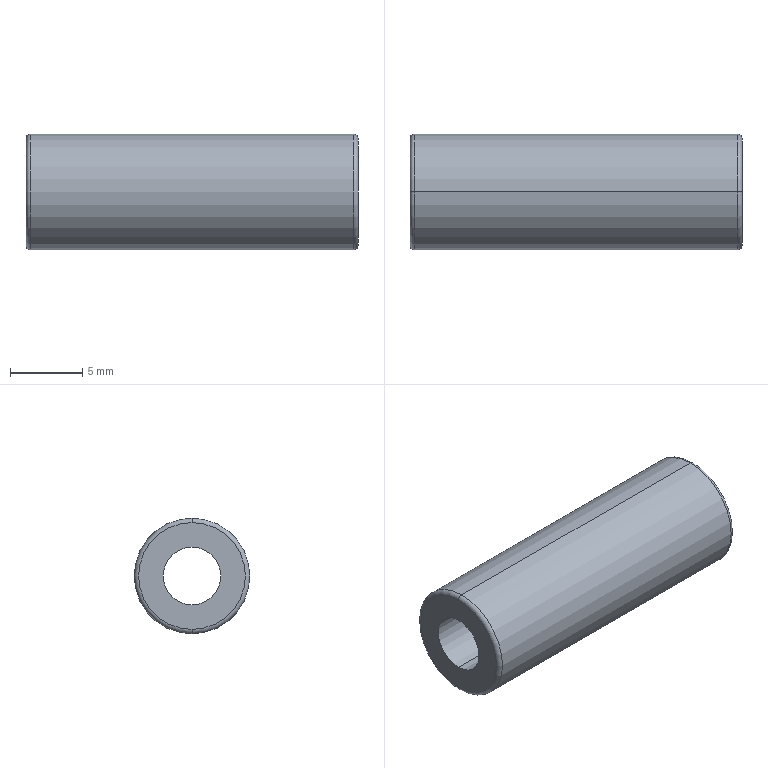Part | SolidWorks | features RefAxis 3, 3DProfileFeature 1, Revolution 1 | 1 solid | 10 faces | box 23 x 8 x 8 mm | volume 866.125 mm3 | torus 4 | cylinder 4 | plane 2 | commonest cylinder face diameters 4 x2 8 x2
STEP:
#1=CARTESIAN_POINT('',(0.3,0.,4.));
#2=VERTEX_POINT('',#1);
#3=CARTESIAN_POINT('',(0.3,0.,-4.));
#4=VERTEX_POINT('',#3);
#5=CARTESIAN_POINT('',(0.3,0.,0.));
#6=DIRECTION('',(-1.,0.,0.));
#7=DIRECTION('',(0.,0.,1.));
#8=AXIS2_PLACEMENT_3D('',#5,#6,#7);
#9=CIRCLE('',#8,4.);
#10=EDGE_CURVE('',#2,#4,#9,.T.);
#11=ORIENTED_EDGE('',*,*,#10,.T.);
#12=CARTESIAN_POINT('',(0.,0.,-3.7));
#13=VERTEX_POINT('',#12);
#14=CARTESIAN_POINT('',(0.3,0.,-3.7));
#15=DIRECTION('',(0.,1.,0.));
#16=DIRECTION('',(0.,0.,1.));
#17=AXIS2_PLACEMENT_3D('',#14,#15,#16);
#18=CIRCLE('',#17,0.3);
#19=EDGE_CURVE('',#4,#13,#18,.T.);
#20=ORIENTED_EDGE('',*,*,#19,.T.);
#21=CARTESIAN_POINT('',(0.,0.,3.7));
#22=VERTEX_POINT('',#21);
#23=CARTESIAN_POINT('',(0.,0.,0.));
#24=DIRECTION('',(-1.,0.,0.));
#25=DIRECTION('',(0.,0.,1.));
#26=AXIS2_PLACEMENT_3D('',#23,#24,#25);
#27=CIRCLE('',#26,3.7);
#28=EDGE_CURVE('',#22,#13,#27,.T.);
#29=ORIENTED_EDGE('',*,*,#28,.F.);
#30=CARTESIAN_POINT('',(0.3,0.,3.7));
#31=DIRECTION('',(0.,-1.,0.));
#32=DIRECTION('',(0.,0.,-1.));
#33=AXIS2_PLACEMENT_3D('',#30,#31,#32);
#34=CIRCLE('',#33,0.3);
#35=EDGE_CURVE('',#2,#22,#34,.T.);
#36=ORIENTED_EDGE('',*,*,#35,.F.);
#37=EDGE_LOOP('',(#11,#20,#29,#36));
#38=FACE_OUTER_BOUND('',#37,.T.);
#39=CARTESIAN_POINT('',(0.3,0.,0.));
#40=DIRECTION('',(-1.,0.,0.));
#41=DIRECTION('',(0.,0.,1.));
#42=AXIS2_PLACEMENT_3D('',#39,#40,#41);
#43=TOROIDAL_SURFACE('',#42,3.7,0.3);
#44=ADVANCED_FACE('',(#38),#43,.T.);
#45=CARTESIAN_POINT('',(22.7,0.,4.));
#46=VERTEX_POINT('',#45);
#47=CARTESIAN_POINT('',(22.7,0.,-4.));
#48=VERTEX_POINT('',#47);
#49=CARTESIAN_POINT('',(22.7,0.,0.));
#50=DIRECTION('',(-1.,0.,0.));
#51=DIRECTION('',(0.,0.,1.));
#52=AXIS2_PLACEMENT_3D('',#49,#50,#51);
#53=CIRCLE('',#52,4.);
#54=EDGE_CURVE('',#46,#48,#53,.T.);
#55=ORIENTED_EDGE('',*,*,#54,.T.);
#56=CARTESIAN_POINT('',(50.,0.,-4.));
#57=DIRECTION('',(-1.,0.,0.));
#58=VECTOR('',#57,1000.);
#59=LINE('',#56,#58);
#60=EDGE_CURVE('',#48,#4,#59,.T.);
#61=ORIENTED_EDGE('',*,*,#60,.T.);
#62=ORIENTED_EDGE('',*,*,#10,.F.);
#63=CARTESIAN_POINT('',(50.,0.,4.));
#64=DIRECTION('',(-1.,0.,0.));
#65=VECTOR('',#64,1000.);
#66=LINE('',#63,#65);
#67=EDGE_CURVE('',#46,#2,#66,.T.);
#68=ORIENTED_EDGE('',*,*,#67,.F.);
#69=EDGE_LOOP('',(#55,#61,#62,#68));
#70=FACE_OUTER_BOUND('',#69,.T.);
#71=CARTESIAN_POINT('',(50.,0.,0.));
#72=DIRECTION('',(-1.,0.,0.));
#73=DIRECTION('',(0.,0.,1.));
#74=AXIS2_PLACEMENT_3D('',#71,#72,#73);
#75=CYLINDRICAL_SURFACE('',#74,4.);
#76=ADVANCED_FACE('',(#70),#75,.T.);
#77=CARTESIAN_POINT('',(23.,0.,3.7));
#78=VERTEX_POINT('',#77);
#79=CARTESIAN_POINT('',(23.,0.,-3.7));
#80=VERTEX_POINT('',#79);
#81=CARTESIAN_POINT('',(23.,0.,0.));
#82=DIRECTION('',(-1.,0.,0.));
#83=DIRECTION('',(0.,0.,1.));
#84=AXIS2_PLACEMENT_3D('',#81,#82,#83);
#85=CIRCLE('',#84,3.7);
#86=EDGE_CURVE('',#78,#80,#85,.T.);
#87=ORIENTED_EDGE('',*,*,#86,.T.);
#88=CARTESIAN_POINT('',(22.7,0.,-3.7));
#89=DIRECTION('',(0.,1.,0.));
#90=DIRECTION('',(0.,0.,1.));
#91=AXIS2_PLACEMENT_3D('',#88,#89,#90);
#92=CIRCLE('',#91,0.3);
#93=EDGE_CURVE('',#80,#48,#92,.T.);
#94=ORIENTED_EDGE('',*,*,#93,.T.);
#95=ORIENTED_EDGE('',*,*,#54,.F.);
#96=CARTESIAN_POINT('',(22.7,0.,3.7));
#97=DIRECTION('',(0.,-1.,0.));
#98=DIRECTION('',(0.,0.,-1.));
#99=AXIS2_PLACEMENT_3D('',#96,#97,#98);
#100=CIRCLE('',#99,0.3);
#101=EDGE_CURVE('',#78,#46,#100,.T.);
#102=ORIENTED_EDGE('',*,*,#101,.F.);
#103=EDGE_LOOP('',(#87,#94,#95,#102));
#104=FACE_OUTER_BOUND('',#103,.T.);
#105=CARTESIAN_POINT('',(22.7,0.,0.));
#106=DIRECTION('',(-1.,0.,0.));
#107=DIRECTION('',(0.,0.,1.));
#108=AXIS2_PLACEMENT_3D('',#105,#106,#107);
#109=TOROIDAL_SURFACE('',#108,3.7,0.3);
#110=ADVANCED_FACE('',(#104),#109,.T.);
#111=CARTESIAN_POINT('',(23.,0.,-2.));
#112=VERTEX_POINT('',#111);
#113=CARTESIAN_POINT('',(23.,0.,2.));
#114=VERTEX_POINT('',#113);
#115=CARTESIAN_POINT('',(23.,0.,0.));
#116=DIRECTION('',(-1.,0.,0.));
#117=DIRECTION('',(0.,0.,1.));
#118=AXIS2_PLACEMENT_3D('',#115,#116,#117);
#119=CIRCLE('',#118,2.);
#120=EDGE_CURVE('',#112,#114,#119,.T.);
#121=ORIENTED_EDGE('',*,*,#120,.F.);
#122=CARTESIAN_POINT('',(0.,0.,-2.));
#123=VERTEX_POINT('',#122);
#124=CARTESIAN_POINT('',(50.,0.,-2.));
#125=DIRECTION('',(-1.,0.,0.));
#126=VECTOR('',#125,1000.);
#127=LINE('',#124,#126);
#128=EDGE_CURVE('',#112,#123,#127,.T.);
#129=ORIENTED_EDGE('',*,*,#128,.T.);
#130=CARTESIAN_POINT('',(0.,0.,2.));
#131=VERTEX_POINT('',#130);
#132=CARTESIAN_POINT('',(0.,0.,0.));
#133=DIRECTION('',(-1.,0.,0.));
#134=DIRECTION('',(0.,0.,1.));
#135=AXIS2_PLACEMENT_3D('',#132,#133,#134);
#136=CIRCLE('',#135,2.);
#137=EDGE_CURVE('',#123,#131,#136,.T.);
#138=ORIENTED_EDGE('',*,*,#137,.T.);
#139=CARTESIAN_POINT('',(50.,0.,2.));
#140=DIRECTION('',(-1.,0.,0.));
#141=VECTOR('',#140,1000.);
#142=LINE('',#139,#141);
#143=EDGE_CURVE('',#114,#131,#142,.T.);
#144=ORIENTED_EDGE('',*,*,#143,.F.);
#145=EDGE_LOOP('',(#121,#129,#138,#144));
#146=FACE_OUTER_BOUND('',#145,.T.);
#147=CARTESIAN_POINT('',(50.,0.,0.));
#148=DIRECTION('',(-1.,0.,0.));
#149=DIRECTION('',(0.,0.,1.));
#150=AXIS2_PLACEMENT_3D('',#147,#148,#149);
#151=CYLINDRICAL_SURFACE('',#150,2.);
#152=ADVANCED_FACE('',(#146),#151,.F.);
#153=CARTESIAN_POINT('',(0.,0.,0.));
#154=DIRECTION('',(-1.,0.,0.));
#155=DIRECTION('',(0.,0.,1.));
#156=AXIS2_PLACEMENT_3D('',#153,#154,#155);
#157=CIRCLE('',#156,2.);
#158=EDGE_CURVE('',#131,#123,#157,.T.);
#159=ORIENTED_EDGE('',*,*,#158,.F.);
#160=ORIENTED_EDGE('',*,*,#137,.F.);
#161=EDGE_LOOP('',(#159,#160));
#162=FACE_BOUND('',#161,.T.);
#163=ORIENTED_EDGE('',*,*,#28,.T.);
#164=CARTESIAN_POINT('',(0.,0.,0.));
#165=DIRECTION('',(-1.,0.,0.));
#166=DIRECTION('',(0.,0.,1.));
#167=AXIS2_PLACEMENT_3D('',#164,#165,#166);
#168=CIRCLE('',#167,3.7);
#169=EDGE_CURVE('',#13,#22,#168,.T.);
#170=ORIENTED_EDGE('',*,*,#169,.T.);
#171=EDGE_LOOP('',(#163,#170));
#172=FACE_OUTER_BOUND('',#171,.T.);
#173=CARTESIAN_POINT('',(0.,3.7,0.));
#174=DIRECTION('',(1.,0.,0.));
#175=DIRECTION('',(0.,0.,-1.));
#176=AXIS2_PLACEMENT_3D('',#173,#174,#175);
#177=PLANE('',#176);
#178=ADVANCED_FACE('',(#162,#172),#177,.F.);
#179=ORIENTED_EDGE('',*,*,#128,.F.);
#180=CARTESIAN_POINT('',(23.,0.,0.));
#181=DIRECTION('',(-1.,0.,0.));
#182=DIRECTION('',(0.,0.,1.));
#183=AXIS2_PLACEMENT_3D('',#180,#181,#182);
#184=CIRCLE('',#183,2.);
#185=EDGE_CURVE('',#114,#112,#184,.T.);
#186=ORIENTED_EDGE('',*,*,#185,.F.);
#187=ORIENTED_EDGE('',*,*,#143,.T.);
#188=ORIENTED_EDGE('',*,*,#158,.T.);
#189=EDGE_LOOP('',(#179,#186,#187,#188));
#190=FACE_OUTER_BOUND('',#189,.T.);
#191=CARTESIAN_POINT('',(50.,0.,0.));
#192=DIRECTION('',(-1.,0.,0.));
#193=DIRECTION('',(0.,0.,1.));
#194=AXIS2_PLACEMENT_3D('',#191,#192,#193);
#195=CYLINDRICAL_SURFACE('',#194,2.);
#196=ADVANCED_FACE('',(#190),#195,.F.);
#197=ORIENTED_EDGE('',*,*,#86,.F.);
#198=CARTESIAN_POINT('',(23.,0.,0.));
#199=DIRECTION('',(-1.,0.,0.));
#200=DIRECTION('',(0.,0.,1.));
#201=AXIS2_PLACEMENT_3D('',#198,#199,#200);
#202=CIRCLE('',#201,3.7);
#203=EDGE_CURVE('',#80,#78,#202,.T.);
#204=ORIENTED_EDGE('',*,*,#203,.F.);
#205=EDGE_LOOP('',(#197,#204));
#206=FACE_OUTER_BOUND('',#205,.T.);
#207=ORIENTED_EDGE('',*,*,#185,.T.);
#208=ORIENTED_EDGE('',*,*,#120,.T.);
#209=EDGE_LOOP('',(#207,#208));
#210=FACE_BOUND('',#209,.T.);
#211=CARTESIAN_POINT('',(23.,2.,0.));
#212=DIRECTION('',(-1.,0.,0.));
#213=DIRECTION('',(0.,0.,1.));
#214=AXIS2_PLACEMENT_3D('',#211,#212,#213);
#215=PLANE('',#214);
#216=ADVANCED_FACE('',(#206,#210),#215,.F.);
#217=ORIENTED_EDGE('',*,*,#93,.F.);
#218=ORIENTED_EDGE('',*,*,#203,.T.);
#219=ORIENTED_EDGE('',*,*,#101,.T.);
#220=CARTESIAN_POINT('',(22.7,0.,0.));
#221=DIRECTION('',(-1.,0.,0.));
#222=DIRECTION('',(0.,0.,1.));
#223=AXIS2_PLACEMENT_3D('',#220,#221,#222);
#224=CIRCLE('',#223,4.);
#225=EDGE_CURVE('',#48,#46,#224,.T.);
#226=ORIENTED_EDGE('',*,*,#225,.F.);
#227=EDGE_LOOP('',(#217,#218,#219,#226));
#228=FACE_OUTER_BOUND('',#227,.T.);
#229=CARTESIAN_POINT('',(22.7,0.,0.));
#230=DIRECTION('',(-1.,0.,0.));
#231=DIRECTION('',(0.,0.,1.));
#232=AXIS2_PLACEMENT_3D('',#229,#230,#231);
#233=TOROIDAL_SURFACE('',#232,3.7,0.3);
#234=ADVANCED_FACE('',(#228),#233,.T.);
#235=ORIENTED_EDGE('',*,*,#60,.F.);
#236=ORIENTED_EDGE('',*,*,#225,.T.);
#237=ORIENTED_EDGE('',*,*,#67,.T.);
#238=CARTESIAN_POINT('',(0.3,0.,0.));
#239=DIRECTION('',(-1.,0.,0.));
#240=DIRECTION('',(0.,0.,1.));
#241=AXIS2_PLACEMENT_3D('',#238,#239,#240);
#242=CIRCLE('',#241,4.);
#243=EDGE_CURVE('',#4,#2,#242,.T.);
#244=ORIENTED_EDGE('',*,*,#243,.F.);
#245=EDGE_LOOP('',(#235,#236,#237,#244));
#246=FACE_OUTER_BOUND('',#245,.T.);
#247=CARTESIAN_POINT('',(50.,0.,0.));
#248=DIRECTION('',(-1.,0.,0.));
#249=DIRECTION('',(0.,0.,1.));
#250=AXIS2_PLACEMENT_3D('',#247,#248,#249);
#251=CYLINDRICAL_SURFACE('',#250,4.);
#252=ADVANCED_FACE('',(#246),#251,.T.);
#253=ORIENTED_EDGE('',*,*,#19,.F.);
#254=ORIENTED_EDGE('',*,*,#243,.T.);
#255=ORIENTED_EDGE('',*,*,#35,.T.);
#256=ORIENTED_EDGE('',*,*,#169,.F.);
#257=EDGE_LOOP('',(#253,#254,#255,#256));
#258=FACE_OUTER_BOUND('',#257,.T.);
#259=CARTESIAN_POINT('',(0.3,0.,0.));
#260=DIRECTION('',(-1.,0.,0.));
#261=DIRECTION('',(0.,0.,1.));
#262=AXIS2_PLACEMENT_3D('',#259,#260,#261);
#263=TOROIDAL_SURFACE('',#262,3.7,0.3);
#264=ADVANCED_FACE('',(#258),#263,.T.);
#265=CLOSED_SHELL('',(#44,#76,#110,#152,#178,#196,#216,#234,#252,#264));
#266=MANIFOLD_SOLID_BREP('',#265);
#267=CARTESIAN_POINT('',(0.,0.,0.));
#268=DIRECTION('',(0.,0.,1.));
#269=DIRECTION('',(1.,0.,0.));
#270=AXIS2_PLACEMENT_3D('',#267,#268,#269);
#271=(LENGTH_UNIT()NAMED_UNIT(*)SI_UNIT(.MILLI.,.METRE.));
#272=UNCERTAINTY_MEASURE_WITH_UNIT(LENGTH_MEASURE(0.00001),#271,'','');
#273=(NAMED_UNIT(*)PLANE_ANGLE_UNIT()SI_UNIT($,.RADIAN.));
#274=(NAMED_UNIT(*)SI_UNIT($,.STERADIAN.)SOLID_ANGLE_UNIT());
#275=(GEOMETRIC_REPRESENTATION_CONTEXT(3)GLOBAL_UNCERTAINTY_ASSIGNED_CONTEXT((#272))GLOBAL_UNIT_ASSIGNED_CONTEXT((#271,#273,#274))REPRESENTATION_CONTEXT('',''));
#276=ADVANCED_BREP_SHAPE_REPRESENTATION('',(#266,#270),#275);